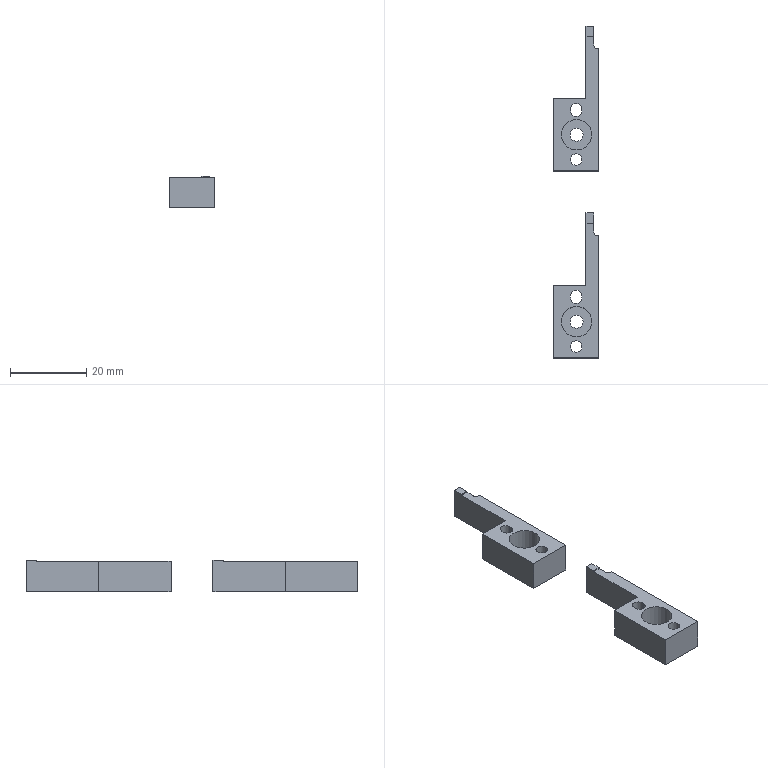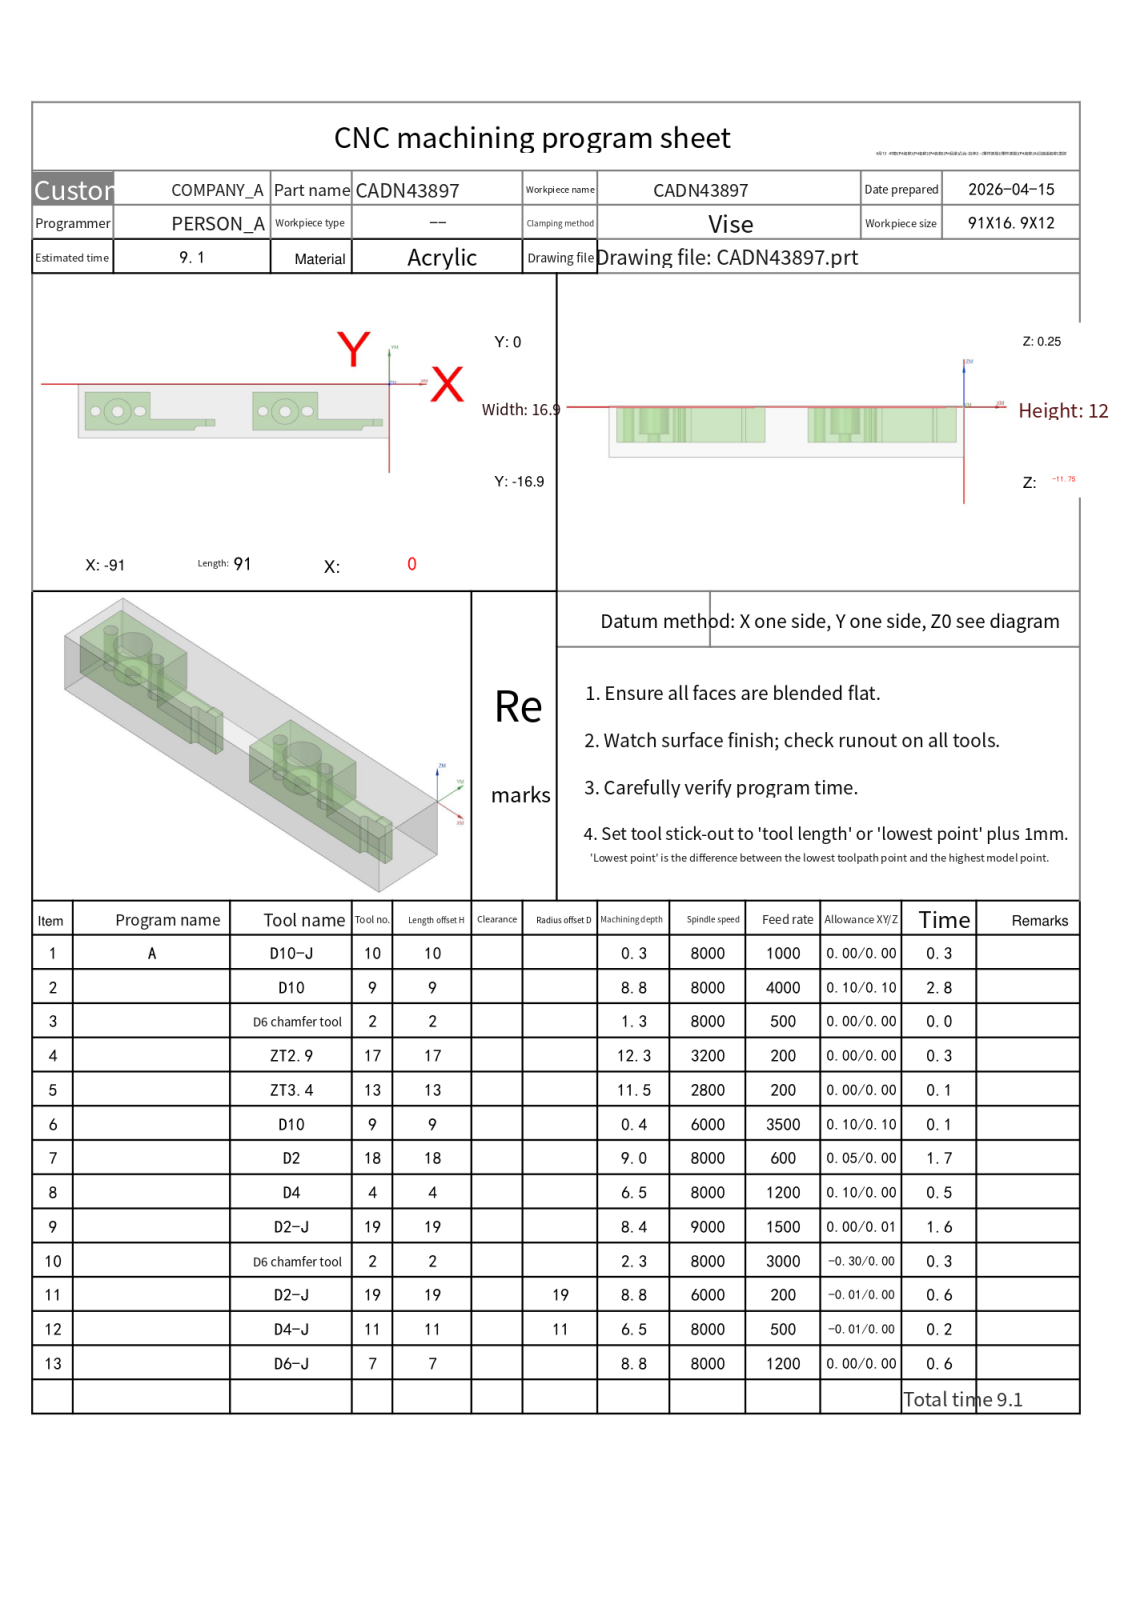NC program | NX | posted by the shop | part box 11.9 x 87 x 8.25 mm
Lines 2111 to 3431 of 9110, first 1079 of 1321 lines:
N7 T18 M06
(D2  D=2. R=0. H=18 ce=0.05 di=0.00)
G00 G90 G54 X-73. Y-8.05 M03 S6000
G43 H18 Z20.
M08
Z.25
G01 X-73.25 Z.244 F600.
G03 X-73.7 Y-8.5 Z.225 I0.0 J-.45
X-73.25 Y-8.95 Z.207 I.45 J0.0
G01 X-72.75 Z.194
G03 X-72.3 Y-8.5 Z.176 I0.0 J.45
X-72.75 Y-8.05 Z.158 I-.45 J0.0
G01 X-73.25 Z.145
G03 X-73.7 Y-8.5 Z.126 I0.0 J-.45
X-73.25 Y-8.95 Z.108 I.45 J0.0
G01 X-72.75 Z.095
G03 X-72.3 Y-8.5 Z.077 I0.0 J.45
X-72.75 Y-8.05 Z.059 I-.45 J0.0
G01 X-73.25 Z.046
G03 X-73.7 Y-8.5 Z.027 I0.0 J-.45
X-73.25 Y-8.95 Z.009 I.45 J0.0
G01 X-72.75 Z-.004
G03 X-72.3 Y-8.5 Z-.022 I0.0 J.45
X-72.75 Y-8.05 Z-.04 I-.45 J0.0
G01 X-73.25 Z-.053
G03 X-73.7 Y-8.5 Z-.071 I0.0 J-.45
X-73.25 Y-8.95 Z-.09 I.45 J0.0
G01 X-72.75 Z-.103
G03 X-72.3 Y-8.5 Z-.121 I0.0 J.45
X-72.75 Y-8.05 Z-.139 I-.45 J0.0
G01 X-73.25 Z-.152
G03 X-73.7 Y-8.5 Z-.17 I0.0 J-.45
X-73.25 Y-8.95 Z-.189 I.45 J0.0
G01 X-72.75 Z-.202
G03 X-72.3 Y-8.5 Z-.22 I0.0 J.45
X-72.75 Y-8.05 Z-.238 I-.45 J0.0
G01 X-73.25 Z-.251
G03 X-73.7 Y-8.5 Z-.269 I0.0 J-.45
X-73.25 Y-8.95 Z-.287 I.45 J0.0
G01 X-72.75 Z-.3
G03 X-72.3 Y-8.5 Z-.319 I0.0 J.45
X-72.75 Y-8.05 Z-.337 I-.45 J0.0
G01 X-73.25 Z-.35
G03 X-73.7 Y-8.5 Z-.368 I0.0 J-.45
X-73.25 Y-8.95 Z-.386 I.45 J0.0
G01 X-72.75 Z-.399
G03 X-72.3 Y-8.5 Z-.418 I0.0 J.45
X-72.75 Y-8.05 Z-.436 I-.45 J0.0
G01 X-73.25 Z-.449
G03 X-73.7 Y-8.5 Z-.467 I0.0 J-.45
X-73.25 Y-8.95 Z-.485 I.45 J0.0
G01 X-72.75 Z-.498
G03 X-72.3 Y-8.5 Z-.516 I0.0 J.45
X-72.75 Y-8.05 Z-.535 I-.45 J0.0
G01 X-73.25 Z-.548
G03 X-73.7 Y-8.5 Z-.566 I0.0 J-.45
X-73.25 Y-8.95 Z-.584 I.45 J0.0
G01 X-72.75 Z-.597
G03 X-72.3 Y-8.5 Z-.615 I0.0 J.45
X-72.75 Y-8.05 Z-.634 I-.45 J0.0
G01 X-73.25 Z-.647
G03 X-73.7 Y-8.5 Z-.665 I0.0 J-.45
X-73.25 Y-8.95 Z-.683 I.45 J0.0
G01 X-72.75 Z-.696
G03 X-72.3 Y-8.5 Z-.714 I0.0 J.45
X-72.75 Y-8.05 Z-.733 I-.45 J0.0
G01 X-73.25 Z-.745
G03 X-73.7 Y-8.5 Z-.764 I0.0 J-.45
X-73.25 Y-8.95 Z-.782 I.45 J0.0
G01 X-72.75 Z-.795
G03 X-72.3 Y-8.5 Z-.813 I0.0 J.45
X-72.75 Y-8.05 Z-.831 I-.45 J0.0
G01 X-73.25 Z-.844
G03 X-73.7 Y-8.5 Z-.863 I0.0 J-.45
X-73.25 Y-8.95 Z-.881 I.45 J0.0
G01 X-72.75 Z-.894
G03 X-72.3 Y-8.5 Z-.912 I0.0 J.45
X-72.75 Y-8.05 Z-.93 I-.45 J0.0
G01 X-73.25 Z-.943
G03 X-73.7 Y-8.5 Z-.962 I0.0 J-.45
X-73.25 Y-8.95 Z-.98 I.45 J0.0
G01 X-72.75 Z-.993
G03 X-72.3 Y-8.5 Z-1.011 I0.0 J.45
X-72.75 Y-8.05 Z-1.029 I-.45 J0.0
G01 X-73.25 Z-1.042
G03 X-73.7 Y-8.5 Z-1.06 I0.0 J-.45
X-73.25 Y-8.95 Z-1.079 I.45 J0.0
G01 X-72.75 Z-1.092
G03 X-72.3 Y-8.5 Z-1.11 I0.0 J.45
X-72.75 Y-8.05 Z-1.128 I-.45 J0.0
G01 X-73.25 Z-1.141
G03 X-73.7 Y-8.5 Z-1.159 I0.0 J-.45
X-73.25 Y-8.95 Z-1.178 I.45 J0.0
G01 X-72.75 Z-1.191
G03 X-72.3 Y-8.5 Z-1.209 I0.0 J.45
X-72.75 Y-8.05 Z-1.227 I-.45 J0.0
G01 X-73.25 Z-1.24
G03 X-73.7 Y-8.5 Z-1.258 I0.0 J-.45
X-73.25 Y-8.95 Z-1.277 I.45 J0.0
G01 X-72.75 Z-1.289
G03 X-72.3 Y-8.5 Z-1.308 I0.0 J.45
X-72.75 Y-8.05 Z-1.326 I-.45 J0.0
G01 X-73.25 Z-1.339
G03 X-73.7 Y-8.5 Z-1.357 I0.0 J-.45
X-73.25 Y-8.95 Z-1.375 I.45 J0.0
G01 X-72.75 Z-1.388
G03 X-72.3 Y-8.5 Z-1.407 I0.0 J.45
X-72.75 Y-8.05 Z-1.425 I-.45 J0.0
G01 X-73.25 Z-1.438
G03 X-73.7 Y-8.5 Z-1.456 I0.0 J-.45
X-73.25 Y-8.95 Z-1.474 I.45 J0.0
G01 X-72.75 Z-1.487
G03 X-72.3 Y-8.5 Z-1.505 I0.0 J.45
X-72.75 Y-8.05 Z-1.524 I-.45 J0.0
G01 X-73.25 Z-1.537
G03 X-73.7 Y-8.5 Z-1.555 I0.0 J-.45
X-73.25 Y-8.95 Z-1.573 I.45 J0.0
G01 X-72.75 Z-1.586
G03 X-72.3 Y-8.5 Z-1.604 I0.0 J.45
X-72.75 Y-8.05 Z-1.623 I-.45 J0.0
G01 X-73.25 Z-1.636
G03 X-73.7 Y-8.5 Z-1.654 I0.0 J-.45
X-73.25 Y-8.95 Z-1.672 I.45 J0.0
G01 X-72.75 Z-1.685
G03 X-72.3 Y-8.5 Z-1.703 I0.0 J.45
X-72.75 Y-8.05 Z-1.722 I-.45 J0.0
G01 X-73.25 Z-1.734
G03 X-73.7 Y-8.5 Z-1.753 I0.0 J-.45
X-73.25 Y-8.95 Z-1.771 I.45 J0.0
G01 X-72.75 Z-1.784
G03 X-72.3 Y-8.5 Z-1.802 I0.0 J.45
X-72.75 Y-8.05 Z-1.82 I-.45 J0.0
G01 X-73.25 Z-1.833
G03 X-73.7 Y-8.5 Z-1.852 I0.0 J-.45
X-73.25 Y-8.95 Z-1.87 I.45 J0.0
G01 X-72.75 Z-1.883
G03 X-72.3 Y-8.5 Z-1.901 I0.0 J.45
X-72.75 Y-8.05 Z-1.919 I-.45 J0.0
G01 X-73.25 Z-1.932
G03 X-73.7 Y-8.5 Z-1.951 I0.0 J-.45
X-73.25 Y-8.95 Z-1.969 I.45 J0.0
G01 X-72.75 Z-1.982
G03 X-72.3 Y-8.5 Z-2. I0.0 J.45
X-72.75 Y-8.05 Z-2.018 I-.45 J0.0
G01 X-73.25 Z-2.031
G03 X-73.7 Y-8.5 Z-2.049 I0.0 J-.45
X-73.25 Y-8.95 Z-2.068 I.45 J0.0
G01 X-72.75 Z-2.081
G03 X-72.3 Y-8.5 Z-2.099 I0.0 J.45
X-72.75 Y-8.05 Z-2.117 I-.45 J0.0
G01 X-73.25 Z-2.13
G03 X-73.7 Y-8.5 Z-2.148 I0.0 J-.45
X-73.25 Y-8.95 Z-2.167 I.45 J0.0
G01 X-72.75 Z-2.18
G03 X-72.3 Y-8.5 Z-2.198 I0.0 J.45
X-72.75 Y-8.05 Z-2.216 I-.45 J0.0
G01 X-73.25 Z-2.229
G03 X-73.7 Y-8.5 Z-2.247 I0.0 J-.45
X-73.25 Y-8.95 Z-2.266 I.45 J0.0
G01 X-72.75 Z-2.278
G03 X-72.3 Y-8.5 Z-2.297 I0.0 J.45
X-72.75 Y-8.05 Z-2.315 I-.45 J0.0
G01 X-73.25 Z-2.328
G03 X-73.7 Y-8.5 Z-2.346 I0.0 J-.45
X-73.25 Y-8.95 Z-2.364 I.45 J0.0
G01 X-72.75 Z-2.377
G03 X-72.3 Y-8.5 Z-2.396 I0.0 J.45
X-72.75 Y-8.05 Z-2.414 I-.45 J0.0
G01 X-73.25 Z-2.427
G03 X-73.7 Y-8.5 Z-2.445 I0.0 J-.45
X-73.25 Y-8.95 Z-2.463 I.45 J0.0
G01 X-72.75 Z-2.476
G03 X-72.3 Y-8.5 Z-2.495 I0.0 J.45
X-72.75 Y-8.05 Z-2.513 I-.45 J0.0
G01 X-73.25 Z-2.526
G03 X-73.7 Y-8.5 Z-2.544 I0.0 J-.45
X-73.25 Y-8.95 Z-2.562 I.45 J0.0
G01 X-72.75 Z-2.575
G03 X-72.3 Y-8.5 Z-2.593 I0.0 J.45
X-72.75 Y-8.05 Z-2.612 I-.45 J0.0
G01 X-73.25 Z-2.625
G03 X-73.7 Y-8.5 Z-2.643 I0.0 J-.45
X-73.25 Y-8.95 Z-2.661 I.45 J0.0
G01 X-72.75 Z-2.674
G03 X-72.3 Y-8.5 Z-2.692 I0.0 J.45
X-72.75 Y-8.05 Z-2.711 I-.45 J0.0
G01 X-73.25 Z-2.723
G03 X-73.7 Y-8.5 Z-2.742 I0.0 J-.45
X-73.25 Y-8.95 Z-2.76 I.45 J0.0
G01 X-72.75 Z-2.773
G03 X-72.3 Y-8.5 Z-2.791 I0.0 J.45
X-72.75 Y-8.05 Z-2.809 I-.45 J0.0
G01 X-73.25 Z-2.822
G03 X-73.7 Y-8.5 Z-2.841 I0.0 J-.45
X-73.25 Y-8.95 Z-2.859 I.45 J0.0
G01 X-72.75 Z-2.872
G03 X-72.3 Y-8.5 Z-2.89 I0.0 J.45
X-72.75 Y-8.05 Z-2.908 I-.45 J0.0
G01 X-73.25 Z-2.921
G03 X-73.7 Y-8.5 Z-2.94 I0.0 J-.45
X-73.25 Y-8.95 Z-2.958 I.45 J0.0
G01 X-72.75 Z-2.971
G03 X-72.3 Y-8.5 Z-2.989 I0.0 J.45
X-72.75 Y-8.05 Z-3.007 I-.45 J0.0
G01 X-73.25 Z-3.02
G03 X-73.7 Y-8.5 Z-3.038 I0.0 J-.45
X-73.25 Y-8.95 Z-3.057 I.45 J0.0
G01 X-72.75 Z-3.07
G03 X-72.3 Y-8.5 Z-3.088 I0.0 J.45
X-72.75 Y-8.05 Z-3.106 I-.45 J0.0
G01 X-73.25 Z-3.119
G03 X-73.7 Y-8.5 Z-3.137 I0.0 J-.45
X-73.25 Y-8.95 Z-3.156 I.45 J0.0
G01 X-72.75 Z-3.169
G03 X-72.3 Y-8.5 Z-3.187 I0.0 J.45
X-72.75 Y-8.05 Z-3.205 I-.45 J0.0
G01 X-73.25 Z-3.218
G03 X-73.7 Y-8.5 Z-3.236 I0.0 J-.45
X-73.25 Y-8.95 Z-3.255 I.45 J0.0
G01 X-72.75 Z-3.267
G03 X-72.3 Y-8.5 Z-3.286 I0.0 J.45
X-72.75 Y-8.05 Z-3.304 I-.45 J0.0
G01 X-73.25 Z-3.317
G03 X-73.7 Y-8.5 Z-3.335 I0.0 J-.45
X-73.25 Y-8.95 Z-3.353 I.45 J0.0
G01 X-72.75 Z-3.366
G03 X-72.3 Y-8.5 Z-3.385 I0.0 J.45
X-72.75 Y-8.05 Z-3.403 I-.45 J0.0
G01 X-73.25 Z-3.416
G03 X-73.7 Y-8.5 Z-3.434 I0.0 J-.45
X-73.25 Y-8.95 Z-3.452 I.45 J0.0
G01 X-72.75 Z-3.465
G03 X-72.3 Y-8.5 Z-3.484 I0.0 J.45
X-72.75 Y-8.05 Z-3.502 I-.45 J0.0
G01 X-73.25 Z-3.515
G03 X-73.7 Y-8.5 Z-3.533 I0.0 J-.45
X-73.25 Y-8.95 Z-3.551 I.45 J0.0
G01 X-72.75 Z-3.564
G03 X-72.3 Y-8.5 Z-3.582 I0.0 J.45
X-72.75 Y-8.05 Z-3.601 I-.45 J0.0
G01 X-73.25 Z-3.614
G03 X-73.7 Y-8.5 Z-3.632 I0.0 J-.45
X-73.25 Y-8.95 Z-3.65 I.45 J0.0
G01 X-72.75 Z-3.663
G03 X-72.3 Y-8.5 Z-3.681 I0.0 J.45
X-72.75 Y-8.05 Z-3.7 I-.45 J0.0
G01 X-73.25 Z-3.713
G03 X-73.7 Y-8.5 Z-3.731 I0.0 J-.45
X-73.25 Y-8.95 Z-3.749 I.45 J0.0
G01 X-72.75 Z-3.762
G03 X-72.3 Y-8.5 Z-3.78 I0.0 J.45
X-72.75 Y-8.05 Z-3.798 I-.45 J0.0
G01 X-73.25 Z-3.811
G03 X-73.7 Y-8.5 Z-3.83 I0.0 J-.45
X-73.25 Y-8.95 Z-3.848 I.45 J0.0
G01 X-72.75 Z-3.861
G03 X-72.3 Y-8.5 Z-3.879 I0.0 J.45
X-72.75 Y-8.05 Z-3.897 I-.45 J0.0
G01 X-73.25 Z-3.91
G03 X-73.7 Y-8.5 Z-3.929 I0.0 J-.45
X-73.25 Y-8.95 Z-3.947 I.45 J0.0
G01 X-72.75 Z-3.96
G03 X-72.3 Y-8.5 Z-3.978 I0.0 J.45
X-72.75 Y-8.05 Z-3.996 I-.45 J0.0
G01 X-73.25 Z-4.009
G03 X-73.7 Y-8.5 Z-4.027 I0.0 J-.45
X-73.25 Y-8.95 Z-4.046 I.45 J0.0
G01 X-72.75 Z-4.059
G03 X-72.3 Y-8.5 Z-4.077 I0.0 J.45
X-72.75 Y-8.05 Z-4.095 I-.45 J0.0
G01 X-73.25 Z-4.108
G03 X-73.7 Y-8.5 Z-4.126 I0.0 J-.45
X-73.25 Y-8.95 Z-4.145 I.45 J0.0
G01 X-72.75 Z-4.158
G03 X-72.3 Y-8.5 Z-4.176 I0.0 J.45
X-72.75 Y-8.05 Z-4.194 I-.45 J0.0
G01 X-73.25 Z-4.207
G03 X-73.7 Y-8.5 Z-4.225 I0.0 J-.45
X-73.25 Y-8.95 Z-4.244 I.45 J0.0
G01 X-72.75 Z-4.256
G03 X-72.3 Y-8.5 Z-4.275 I0.0 J.45
X-72.75 Y-8.05 Z-4.293 I-.45 J0.0
G01 X-73.25 Z-4.306
G03 X-73.7 Y-8.5 Z-4.324 I0.0 J-.45
X-73.25 Y-8.95 Z-4.342 I.45 J0.0
G01 X-72.75 Z-4.355
G03 X-72.3 Y-8.5 Z-4.374 I0.0 J.45
X-72.75 Y-8.05 Z-4.392 I-.45 J0.0
G01 X-73.25 Z-4.405
G03 X-73.7 Y-8.5 Z-4.423 I0.0 J-.45
X-73.25 Y-8.95 Z-4.441 I.45 J0.0
G01 X-72.75 Z-4.454
G03 X-72.3 Y-8.5 Z-4.473 I0.0 J.45
X-72.75 Y-8.05 Z-4.491 I-.45 J0.0
G01 X-73.25 Z-4.504
G03 X-73.7 Y-8.5 Z-4.522 I0.0 J-.45
X-73.25 Y-8.95 Z-4.54 I.45 J0.0
G01 X-72.75 Z-4.553
G03 X-72.3 Y-8.5 Z-4.571 I0.0 J.45
X-72.75 Y-8.05 Z-4.59 I-.45 J0.0
G01 X-73.25 Z-4.603
G03 X-73.7 Y-8.5 Z-4.621 I0.0 J-.45
X-73.25 Y-8.95 Z-4.639 I.45 J0.0
G01 X-72.75 Z-4.652
G03 X-72.3 Y-8.5 Z-4.67 I0.0 J.45
X-72.75 Y-8.05 Z-4.689 I-.45 J0.0
G01 X-73.25 Z-4.702
G03 X-73.7 Y-8.5 Z-4.72 I0.0 J-.45
X-73.25 Y-8.95 Z-4.738 I.45 J0.0
G01 X-72.75 Z-4.751
G03 X-72.3 Y-8.5 Z-4.769 I0.0 J.45
X-72.75 Y-8.05 Z-4.787 I-.45 J0.0
G01 X-73.25 Z-4.8
G03 X-73.7 Y-8.5 Z-4.819 I0.0 J-.45
X-73.25 Y-8.95 Z-4.837 I.45 J0.0
G01 X-72.75 Z-4.85
G03 X-72.3 Y-8.5 Z-4.868 I0.0 J.45
X-72.75 Y-8.05 Z-4.886 I-.45 J0.0
G01 X-73.25 Z-4.899
G03 X-73.7 Y-8.5 Z-4.918 I0.0 J-.45
X-73.25 Y-8.95 Z-4.936 I.45 J0.0
G01 X-72.75 Z-4.949
G03 X-72.3 Y-8.5 Z-4.967 I0.0 J.45
X-72.75 Y-8.05 Z-4.985 I-.45 J0.0
G01 X-73.25 Z-4.998
G03 X-73.7 Y-8.5 Z-5.016 I0.0 J-.45
X-73.25 Y-8.95 Z-5.035 I.45 J0.0
G01 X-72.75 Z-5.048
G03 X-72.3 Y-8.5 Z-5.066 I0.0 J.45
X-72.75 Y-8.05 Z-5.084 I-.45 J0.0
G01 X-73.25 Z-5.097
G03 X-73.7 Y-8.5 Z-5.115 I0.0 J-.45
X-73.25 Y-8.95 Z-5.134 I.45 J0.0
G01 X-72.75 Z-5.147
G03 X-72.3 Y-8.5 Z-5.165 I0.0 J.45
X-72.75 Y-8.05 Z-5.183 I-.45 J0.0
G01 X-73.25 Z-5.196
G03 X-73.7 Y-8.5 Z-5.214 I0.0 J-.45
X-73.25 Y-8.95 Z-5.233 I.45 J0.0
G01 X-72.75 Z-5.245
G03 X-72.3 Y-8.5 Z-5.264 I0.0 J.45
X-72.75 Y-8.05 Z-5.282 I-.45 J0.0
G01 X-73.25 Z-5.295
G03 X-73.7 Y-8.5 Z-5.313 I0.0 J-.45
X-73.25 Y-8.95 Z-5.331 I.45 J0.0
G01 X-72.75 Z-5.344
G03 X-72.3 Y-8.5 Z-5.363 I0.0 J.45
X-72.75 Y-8.05 Z-5.381 I-.45 J0.0
G01 X-73.25 Z-5.394
G03 X-73.7 Y-8.5 Z-5.412 I0.0 J-.45
X-73.25 Y-8.95 Z-5.43 I.45 J0.0
G01 X-72.75 Z-5.443
G03 X-72.3 Y-8.5 Z-5.462 I0.0 J.45
X-72.75 Y-8.05 Z-5.48 I-.45 J0.0
G01 X-73.25 Z-5.493
G03 X-73.7 Y-8.5 Z-5.511 I0.0 J-.45
X-73.25 Y-8.95 Z-5.529 I.45 J0.0
G01 X-72.75 Z-5.542
G03 X-72.3 Y-8.5 Z-5.56 I0.0 J.45
X-72.75 Y-8.05 Z-5.579 I-.45 J0.0
G01 X-73.25 Z-5.592
G03 X-73.7 Y-8.5 Z-5.61 I0.0 J-.45
X-73.25 Y-8.95 Z-5.628 I.45 J0.0
G01 X-72.75 Z-5.641
G03 X-72.3 Y-8.5 Z-5.659 I0.0 J.45
X-72.75 Y-8.05 Z-5.678 I-.45 J0.0
G01 X-73.25 Z-5.691
G03 X-73.7 Y-8.5 Z-5.709 I0.0 J-.45
X-73.25 Y-8.95 Z-5.727 I.45 J0.0
G01 X-72.75 Z-5.74
G03 X-72.3 Y-8.5 Z-5.758 I0.0 J.45
X-72.75 Y-8.05 Z-5.777 I-.45 J0.0
G01 X-73.25 Z-5.789
G03 X-73.7 Y-8.5 Z-5.808 I0.0 J-.45
X-73.25 Y-8.95 Z-5.826 I.45 J0.0
G01 X-72.75 Z-5.839
G03 X-72.3 Y-8.5 Z-5.857 I0.0 J.45
X-72.75 Y-8.05 Z-5.875 I-.45 J0.0
G01 X-73.25 Z-5.888
G03 X-73.7 Y-8.5 Z-5.907 I0.0 J-.45
X-73.25 Y-8.95 Z-5.925 I.45 J0.0
G01 X-72.75 Z-5.938
G03 X-72.3 Y-8.5 Z-5.956 I0.0 J.45
X-72.75 Y-8.05 Z-5.974 I-.45 J0.0
G01 X-73.25 Z-5.987
G03 X-73.7 Y-8.5 Z-6.005 I0.0 J-.45
X-73.25 Y-8.95 Z-6.024 I.45 J0.0
G01 X-72.75 Z-6.037
G03 X-72.3 Y-8.5 Z-6.055 I0.0 J.45
X-72.75 Y-8.05 Z-6.073 I-.45 J0.0
G01 X-73.25 Z-6.086
G03 X-73.7 Y-8.5 Z-6.104 I0.0 J-.45
X-73.25 Y-8.95 Z-6.123 I.45 J0.0
G01 X-72.75 Z-6.136
G03 X-72.3 Y-8.5 Z-6.154 I0.0 J.45
X-72.75 Y-8.05 Z-6.172 I-.45 J0.0
G01 X-73.25 Z-6.185
G03 X-73.7 Y-8.5 Z-6.203 I0.0 J-.45
X-73.25 Y-8.95 Z-6.222 I.45 J0.0
G01 X-72.75 Z-6.234
G03 X-72.3 Y-8.5 Z-6.253 I0.0 J.45
X-72.75 Y-8.05 Z-6.271 I-.45 J0.0
G01 X-73.25 Z-6.284
G03 X-73.7 Y-8.5 Z-6.302 I0.0 J-.45
X-73.25 Y-8.95 Z-6.32 I.45 J0.0
G01 X-72.75 Z-6.333
G03 X-72.3 Y-8.5 Z-6.352 I0.0 J.45
X-72.75 Y-8.05 Z-6.37 I-.45 J0.0
G01 X-73.25 Z-6.383
G03 X-73.7 Y-8.5 Z-6.401 I0.0 J-.45
X-73.25 Y-8.95 Z-6.419 I.45 J0.0
G01 X-72.75 Z-6.432
G03 X-72.3 Y-8.5 Z-6.451 I0.0 J.45
X-72.75 Y-8.05 Z-6.469 I-.45 J0.0
G01 X-73.25 Z-6.482
G03 X-73.7 Y-8.5 Z-6.5 I0.0 J-.45
X-73.25 Y-8.95 Z-6.518 I.45 J0.0
G01 X-72.75 Z-6.531
G03 X-72.3 Y-8.5 Z-6.549 I0.0 J.45
X-72.75 Y-8.05 Z-6.568 I-.45 J0.0
G01 X-73.25 Z-6.581
G03 X-73.7 Y-8.5 Z-6.599 I0.0 J-.45
X-73.25 Y-8.95 Z-6.617 I.45 J0.0
G01 X-72.75 Z-6.63
G03 X-72.3 Y-8.5 Z-6.648 I0.0 J.45
X-72.75 Y-8.05 Z-6.667 I-.45 J0.0
G01 X-73.25 Z-6.68
G03 X-73.7 Y-8.5 Z-6.698 I0.0 J-.45
X-73.25 Y-8.95 Z-6.716 I.45 J0.0
G01 X-72.75 Z-6.729
G03 X-72.3 Y-8.5 Z-6.747 I0.0 J.45
X-72.75 Y-8.05 Z-6.766 I-.45 J0.0
G01 X-73.25 Z-6.778
G03 X-73.7 Y-8.5 Z-6.797 I0.0 J-.45
X-73.25 Y-8.95 Z-6.815 I.45 J0.0
G01 X-72.75 Z-6.828
G03 X-72.3 Y-8.5 Z-6.846 I0.0 J.45
X-72.75 Y-8.05 Z-6.864 I-.45 J0.0
G01 X-73.25 Z-6.877
G03 X-73.7 Y-8.5 Z-6.896 I0.0 J-.45
X-73.25 Y-8.95 Z-6.914 I.45 J0.0
G01 X-72.75 Z-6.927
G03 X-72.3 Y-8.5 Z-6.945 I0.0 J.45
X-72.75 Y-8.05 Z-6.963 I-.45 J0.0
G01 X-73.25 Z-6.976
G03 X-73.7 Y-8.5 Z-6.995 I0.0 J-.45
X-73.25 Y-8.95 Z-7.013 I.45 J0.0
G01 X-72.75 Z-7.026
G03 X-72.3 Y-8.5 Z-7.044 I0.0 J.45
X-72.75 Y-8.05 Z-7.062 I-.45 J0.0
G01 X-73.25 Z-7.075
G03 X-73.7 Y-8.5 Z-7.093 I0.0 J-.45
X-73.25 Y-8.95 Z-7.112 I.45 J0.0
G01 X-72.75 Z-7.125
G03 X-72.3 Y-8.5 Z-7.143 I0.0 J.45
X-72.75 Y-8.05 Z-7.161 I-.45 J0.0
G01 X-73.25 Z-7.174
G03 X-73.7 Y-8.5 Z-7.192 I0.0 J-.45
X-73.25 Y-8.95 Z-7.211 I.45 J0.0
G01 X-72.75 Z-7.223
G03 X-72.3 Y-8.5 Z-7.242 I0.0 J.45
X-72.75 Y-8.05 Z-7.26 I-.45 J0.0
G01 X-73.25 Z-7.273
G03 X-73.7 Y-8.5 Z-7.291 I0.0 J-.45
X-73.25 Y-8.95 Z-7.309 I.45 J0.0
G01 X-72.75 Z-7.322
G03 X-72.3 Y-8.5 Z-7.341 I0.0 J.45
X-72.75 Y-8.05 Z-7.359 I-.45 J0.0
G01 X-73.25 Z-7.372
G03 X-73.7 Y-8.5 Z-7.39 I0.0 J-.45
X-73.25 Y-8.95 Z-7.408 I.45 J0.0
G01 X-72.75 Z-7.421
G03 X-72.3 Y-8.5 Z-7.44 I0.0 J.45
X-72.75 Y-8.05 Z-7.458 I-.45 J0.0
G01 X-73.25 Z-7.471
G03 X-73.7 Y-8.5 Z-7.489 I0.0 J-.45
X-73.25 Y-8.95 Z-7.507 I.45 J0.0
G01 X-72.75 Z-7.52
G03 X-72.3 Y-8.5 Z-7.538 I0.0 J.45
X-72.75 Y-8.05 Z-7.557 I-.45 J0.0
G01 X-73.25 Z-7.57
G03 X-73.7 Y-8.5 Z-7.588 I0.0 J-.45
X-73.25 Y-8.95 Z-7.606 I.45 J0.0
G01 X-72.75 Z-7.619
G03 X-72.3 Y-8.5 Z-7.637 I0.0 J.45
X-72.75 Y-8.05 Z-7.656 I-.45 J0.0
G01 X-73.25 Z-7.669
G03 X-73.7 Y-8.5 Z-7.687 I0.0 J-.45
X-73.25 Y-8.95 Z-7.705 I.45 J0.0
G01 X-72.75 Z-7.718
G03 X-72.3 Y-8.5 Z-7.736 I0.0 J.45
X-72.75 Y-8.05 Z-7.755 I-.45 J0.0
G01 X-73.25 Z-7.767
G03 X-73.7 Y-8.5 Z-7.786 I0.0 J-.45
X-73.25 Y-8.95 Z-7.804 I.45 J0.0
G01 X-72.75 Z-7.817
G03 X-72.3 Y-8.5 Z-7.835 I0.0 J.45
X-72.75 Y-8.05 Z-7.853 I-.45 J0.0
G01 X-73.25 Z-7.866
G03 X-73.7 Y-8.5 Z-7.885 I0.0 J-.45
X-73.25 Y-8.95 Z-7.903 I.45 J0.0
G01 X-72.75 Z-7.916
G03 X-72.3 Y-8.5 Z-7.934 I0.0 J.45
X-72.75 Y-8.05 Z-7.952 I-.45 J0.0
G01 X-73.25 Z-7.965
G03 X-73.7 Y-8.5 Z-7.984 I0.0 J-.45
X-73.25 Y-8.95 Z-8.002 I.45 J0.0
G01 X-72.75 Z-8.015
G03 X-72.3 Y-8.5 Z-8.033 I0.0 J.45
X-72.75 Y-8.05 Z-8.051 I-.45 J0.0
G01 X-73.25 Z-8.064
G03 X-73.7 Y-8.5 Z-8.082 I0.0 J-.45
X-73.25 Y-8.95 Z-8.101 I.45 J0.0
G01 X-72.75 Z-8.114
G03 X-72.3 Y-8.5 Z-8.132 I0.0 J.45
X-72.75 Y-8.05 Z-8.15 I-.45 J0.0
G01 X-73.25 Z-8.163
G03 X-73.7 Y-8.5 Z-8.181 I0.0 J-.45
X-73.25 Y-8.95 Z-8.2 I.45 J0.0
G01 X-72.75 Z-8.213
G03 X-72.3 Y-8.5 Z-8.231 I0.0 J.45
X-72.75 Y-8.05 Z-8.249 I-.45 J0.0
G01 X-73.25 Z-8.262
G03 X-73.7 Y-8.5 Z-8.28 I0.0 J-.45
X-73.25 Y-8.95 Z-8.298 I.45 J0.0
G01 X-72.75 Z-8.311
G03 X-72.3 Y-8.5 Z-8.33 I0.0 J.45
X-72.75 Y-8.05 Z-8.348 I-.45 J0.0
G01 X-73.25 Z-8.361
G03 X-73.7 Y-8.5 Z-8.379 I0.0 J-.45
X-73.25 Y-8.95 Z-8.397 I.45 J0.0
G01 X-72.75 Z-8.41
G03 X-72.3 Y-8.5 Z-8.429 I0.0 J.45
X-72.75 Y-8.05 Z-8.447 I-.45 J0.0
G01 X-73.25 Z-8.46
G03 X-73.7 Y-8.5 Z-8.478 I0.0 J-.45
X-73.25 Y-8.95 Z-8.496 I.45 J0.0
G01 X-72.75 Z-8.509
G03 X-72.3 Y-8.5 Z-8.527 I0.0 J.45
X-72.75 Y-8.05 Z-8.546 I-.45 J0.0
G01 X-73.25 Z-8.559
G03 X-73.7 Y-8.5 Z-8.577 I0.0 J-.45
X-73.25 Y-8.95 Z-8.595 I.45 J0.0
G01 X-72.75 Z-8.608
G03 X-72.3 Y-8.5 Z-8.626 I0.0 J.45
X-72.75 Y-8.05 Z-8.645 I-.45 J0.0
G01 X-73.25 Z-8.658
G03 X-73.7 Y-8.5 Z-8.676 I0.0 J-.45
X-73.25 Y-8.95 Z-8.694 I.45 J0.0
G01 X-72.75 Z-8.707
G03 X-72.3 Y-8.5 Z-8.725 I0.0 J.45
X-72.75 Y-8.05 Z-8.744 I-.45 J0.0
G01 X-73. Z-8.75
X-73.25
G03 X-73.7 Y-8.5 I0.0 J-.45
X-73.25 Y-8.95 I.45 J0.0
G01 X-72.75
G03 X-72.3 Y-8.5 I0.0 J.45
X-72.75 Y-8.05 I-.45 J0.0
G01 X-73.
X-73.25
G03 X-73.487 Y-8.118 I0.0 J-.45
G01 Z-7.75
G00 Z20.
X-24. Y-8.95
Z.25
G01 X-23.75 Z.244
G03 X-23.3 Y-8.5 Z.225 I0.0 J.45
X-23.75 Y-8.05 Z.207 I-.45 J0.0
G01 X-24.25 Z.194
G03 X-24.7 Y-8.5 Z.176 I0.0 J-.45
X-24.25 Y-8.95 Z.158 I.45 J0.0
G01 X-23.75 Z.145
G03 X-23.3 Y-8.5 Z.126 I0.0 J.45
X-23.75 Y-8.05 Z.108 I-.45 J0.0
G01 X-24.25 Z.095
G03 X-24.7 Y-8.5 Z.077 I0.0 J-.45
X-24.25 Y-8.95 Z.059 I.45 J0.0
G01 X-23.75 Z.046
G03 X-23.3 Y-8.5 Z.027 I0.0 J.45
X-23.75 Y-8.05 Z.009 I-.45 J0.0
G01 X-24.25 Z-.004
G03 X-24.7 Y-8.5 Z-.022 I0.0 J-.45
X-24.25 Y-8.95 Z-.04 I.45 J0.0
G01 X-23.75 Z-.053
G03 X-23.3 Y-8.5 Z-.071 I0.0 J.45
X-23.75 Y-8.05 Z-.09 I-.45 J0.0
G01 X-24.25 Z-.103
G03 X-24.7 Y-8.5 Z-.121 I0.0 J-.45
X-24.25 Y-8.95 Z-.139 I.45 J0.0
G01 X-23.75 Z-.152
G03 X-23.3 Y-8.5 Z-.17 I0.0 J.45
X-23.75 Y-8.05 Z-.189 I-.45 J0.0
G01 X-24.25 Z-.202
G03 X-24.7 Y-8.5 Z-.22 I0.0 J-.45
X-24.25 Y-8.95 Z-.238 I.45 J0.0
G01 X-23.75 Z-.251
G03 X-23.3 Y-8.5 Z-.269 I0.0 J.45
X-23.75 Y-8.05 Z-.287 I-.45 J0.0
G01 X-24.25 Z-.3
G03 X-24.7 Y-8.5 Z-.319 I0.0 J-.45
X-24.25 Y-8.95 Z-.337 I.45 J0.0
G01 X-23.75 Z-.35
G03 X-23.3 Y-8.5 Z-.368 I0.0 J.45
X-23.75 Y-8.05 Z-.386 I-.45 J0.0
G01 X-24.25 Z-.399
G03 X-24.7 Y-8.5 Z-.418 I0.0 J-.45
X-24.25 Y-8.95 Z-.436 I.45 J0.0
G01 X-23.75 Z-.449
G03 X-23.3 Y-8.5 Z-.467 I0.0 J.45
X-23.75 Y-8.05 Z-.485 I-.45 J0.0
G01 X-24.25 Z-.498
G03 X-24.7 Y-8.5 Z-.516 I0.0 J-.45
X-24.25 Y-8.95 Z-.535 I.45 J0.0
G01 X-23.75 Z-.548
G03 X-23.3 Y-8.5 Z-.566 I0.0 J.45
X-23.75 Y-8.05 Z-.584 I-.45 J0.0
G01 X-24.25 Z-.597
G03 X-24.7 Y-8.5 Z-.615 I0.0 J-.45
X-24.25 Y-8.95 Z-.634 I.45 J0.0
G01 X-23.75 Z-.647
G03 X-23.3 Y-8.5 Z-.665 I0.0 J.45
X-23.75 Y-8.05 Z-.683 I-.45 J0.0
G01 X-24.25 Z-.696
G03 X-24.7 Y-8.5 Z-.714 I0.0 J-.45
X-24.25 Y-8.95 Z-.733 I.45 J0.0
G01 X-23.75 Z-.745
G03 X-23.3 Y-8.5 Z-.764 I0.0 J.45
X-23.75 Y-8.05 Z-.782 I-.45 J0.0
G01 X-24.25 Z-.795
G03 X-24.7 Y-8.5 Z-.813 I0.0 J-.45
X-24.25 Y-8.95 Z-.831 I.45 J0.0
G01 X-23.75 Z-.844
G03 X-23.3 Y-8.5 Z-.863 I0.0 J.45
X-23.75 Y-8.05 Z-.881 I-.45 J0.0
G01 X-24.25 Z-.894
G03 X-24.7 Y-8.5 Z-.912 I0.0 J-.45
X-24.25 Y-8.95 Z-.93 I.45 J0.0
G01 X-23.75 Z-.943
G03 X-23.3 Y-8.5 Z-.962 I0.0 J.45
X-23.75 Y-8.05 Z-.98 I-.45 J0.0
G01 X-24.25 Z-.993
G03 X-24.7 Y-8.5 Z-1.011 I0.0 J-.45
X-24.25 Y-8.95 Z-1.029 I.45 J0.0
G01 X-23.75 Z-1.042
G03 X-23.3 Y-8.5 Z-1.06 I0.0 J.45
X-23.75 Y-8.05 Z-1.079 I-.45 J0.0
G01 X-24.25 Z-1.092
G03 X-24.7 Y-8.5 Z-1.11 I0.0 J-.45
X-24.25 Y-8.95 Z-1.128 I.45 J0.0
G01 X-23.75 Z-1.141
G03 X-23.3 Y-8.5 Z-1.159 I0.0 J.45
X-23.75 Y-8.05 Z-1.178 I-.45 J0.0
G01 X-24.25 Z-1.191
G03 X-24.7 Y-8.5 Z-1.209 I0.0 J-.45
X-24.25 Y-8.95 Z-1.227 I.45 J0.0
G01 X-23.75 Z-1.24
G03 X-23.3 Y-8.5 Z-1.258 I0.0 J.45
X-23.75 Y-8.05 Z-1.277 I-.45 J0.0
G01 X-24.25 Z-1.289
G03 X-24.7 Y-8.5 Z-1.308 I0.0 J-.45
X-24.25 Y-8.95 Z-1.326 I.45 J0.0
G01 X-23.75 Z-1.339
G03 X-23.3 Y-8.5 Z-1.357 I0.0 J.45
X-23.75 Y-8.05 Z-1.375 I-.45 J0.0
G01 X-24.25 Z-1.388
G03 X-24.7 Y-8.5 Z-1.407 I0.0 J-.45
X-24.25 Y-8.95 Z-1.425 I.45 J0.0
G01 X-23.75 Z-1.438
G03 X-23.3 Y-8.5 Z-1.456 I0.0 J.45
X-23.75 Y-8.05 Z-1.474 I-.45 J0.0
G01 X-24.25 Z-1.487
G03 X-24.7 Y-8.5 Z-1.505 I0.0 J-.45
X-24.25 Y-8.95 Z-1.524 I.45 J0.0
G01 X-23.75 Z-1.537
G03 X-23.3 Y-8.5 Z-1.555 I0.0 J.45
X-23.75 Y-8.05 Z-1.573 I-.45 J0.0
G01 X-24.25 Z-1.586
G03 X-24.7 Y-8.5 Z-1.604 I0.0 J-.45
X-24.25 Y-8.95 Z-1.623 I.45 J0.0
G01 X-23.75 Z-1.636
G03 X-23.3 Y-8.5 Z-1.654 I0.0 J.45
X-23.75 Y-8.05 Z-1.672 I-.45 J0.0
G01 X-24.25 Z-1.685
G03 X-24.7 Y-8.5 Z-1.703 I0.0 J-.45
X-24.25 Y-8.95 Z-1.722 I.45 J0.0
G01 X-23.75 Z-1.734
G03 X-23.3 Y-8.5 Z-1.753 I0.0 J.45
X-23.75 Y-8.05 Z-1.771 I-.45 J0.0
G01 X-24.25 Z-1.784
G03 X-24.7 Y-8.5 Z-1.802 I0.0 J-.45
X-24.25 Y-8.95 Z-1.82 I.45 J0.0
G01 X-23.75 Z-1.833
G03 X-23.3 Y-8.5 Z-1.852 I0.0 J.45
X-23.75 Y-8.05 Z-1.87 I-.45 J0.0
G01 X-24.25 Z-1.883
G03 X-24.7 Y-8.5 Z-1.901 I0.0 J-.45
X-24.25 Y-8.95 Z-1.919 I.45 J0.0
G01 X-23.75 Z-1.932
G03 X-23.3 Y-8.5 Z-1.951 I0.0 J.45
X-23.75 Y-8.05 Z-1.969 I-.45 J0.0
G01 X-24.25 Z-1.982
G03 X-24.7 Y-8.5 Z-2. I0.0 J-.45
X-24.25 Y-8.95 Z-2.018 I.45 J0.0
G01 X-23.75 Z-2.031
G03 X-23.3 Y-8.5 Z-2.049 I0.0 J.45
X-23.75 Y-8.05 Z-2.068 I-.45 J0.0
G01 X-24.25 Z-2.081
G03 X-24.7 Y-8.5 Z-2.099 I0.0 J-.45
X-24.25 Y-8.95 Z-2.117 I.45 J0.0
G01 X-23.75 Z-2.13
G03 X-23.3 Y-8.5 Z-2.148 I0.0 J.45
X-23.75 Y-8.05 Z-2.167 I-.45 J0.0
G01 X-24.25 Z-2.18
G03 X-24.7 Y-8.5 Z-2.198 I0.0 J-.45
X-24.25 Y-8.95 Z-2.216 I.45 J0.0
G01 X-23.75 Z-2.229
G03 X-23.3 Y-8.5 Z-2.247 I0.0 J.45
X-23.75 Y-8.05 Z-2.266 I-.45 J0.0
G01 X-24.25 Z-2.278
G03 X-24.7 Y-8.5 Z-2.297 I0.0 J-.45
X-24.25 Y-8.95 Z-2.315 I.45 J0.0
G01 X-23.75 Z-2.328
G03 X-23.3 Y-8.5 Z-2.346 I0.0 J.45
X-23.75 Y-8.05 Z-2.364 I-.45 J0.0
G01 X-24.25 Z-2.377
G03 X-24.7 Y-8.5 Z-2.396 I0.0 J-.45
X-24.25 Y-8.95 Z-2.414 I.45 J0.0
G01 X-23.75 Z-2.427
G03 X-23.3 Y-8.5 Z-2.445 I0.0 J.45
X-23.75 Y-8.05 Z-2.463 I-.45 J0.0
G01 X-24.25 Z-2.476
G03 X-24.7 Y-8.5 Z-2.495 I0.0 J-.45
X-24.25 Y-8.95 Z-2.513 I.45 J0.0
G01 X-23.75 Z-2.526
G03 X-23.3 Y-8.5 Z-2.544 I0.0 J.45
X-23.75 Y-8.05 Z-2.562 I-.45 J0.0
G01 X-24.25 Z-2.575
G03 X-24.7 Y-8.5 Z-2.593 I0.0 J-.45
X-24.25 Y-8.95 Z-2.612 I.45 J0.0
G01 X-23.75 Z-2.625
G03 X-23.3 Y-8.5 Z-2.643 I0.0 J.45
X-23.75 Y-8.05 Z-2.661 I-.45 J0.0
G01 X-24.25 Z-2.674
G03 X-24.7 Y-8.5 Z-2.692 I0.0 J-.45
X-24.25 Y-8.95 Z-2.711 I.45 J0.0
G01 X-23.75 Z-2.723
G03 X-23.3 Y-8.5 Z-2.742 I0.0 J.45
X-23.75 Y-8.05 Z-2.76 I-.45 J0.0
G01 X-24.25 Z-2.773
G03 X-24.7 Y-8.5 Z-2.791 I0.0 J-.45
X-24.25 Y-8.95 Z-2.809 I.45 J0.0
G01 X-23.75 Z-2.822
G03 X-23.3 Y-8.5 Z-2.841 I0.0 J.45
X-23.75 Y-8.05 Z-2.859 I-.45 J0.0
G01 X-24.25 Z-2.872
G03 X-24.7 Y-8.5 Z-2.89 I0.0 J-.45
X-24.25 Y-8.95 Z-2.908 I.45 J0.0
G01 X-23.75 Z-2.921
G03 X-23.3 Y-8.5 Z-2.94 I0.0 J.45
X-23.75 Y-8.05 Z-2.958 I-.45 J0.0
G01 X-24.25 Z-2.971
G03 X-24.7 Y-8.5 Z-2.989 I0.0 J-.45
X-24.25 Y-8.95 Z-3.007 I.45 J0.0
G01 X-23.75 Z-3.02
G03 X-23.3 Y-8.5 Z-3.038 I0.0 J.45
X-23.75 Y-8.05 Z-3.057 I-.45 J0.0
G01 X-24.25 Z-3.07
G03 X-24.7 Y-8.5 Z-3.088 I0.0 J-.45
X-24.25 Y-8.95 Z-3.106 I.45 J0.0
G01 X-23.75 Z-3.119
G03 X-23.3 Y-8.5 Z-3.137 I0.0 J.45
X-23.75 Y-8.05 Z-3.156 I-.45 J0.0
G01 X-24.25 Z-3.169
G03 X-24.7 Y-8.5 Z-3.187 I0.0 J-.45
X-24.25 Y-8.95 Z-3.205 I.45 J0.0
G01 X-23.75 Z-3.218
G03 X-23.3 Y-8.5 Z-3.236 I0.0 J.45
X-23.75 Y-8.05 Z-3.255 I-.45 J0.0
G01 X-24.25 Z-3.267
G03 X-24.7 Y-8.5 Z-3.286 I0.0 J-.45
X-24.25 Y-8.95 Z-3.304 I.45 J0.0
G01 X-23.75 Z-3.317
G03 X-23.3 Y-8.5 Z-3.335 I0.0 J.45
X-23.75 Y-8.05 Z-3.353 I-.45 J0.0
G01 X-24.25 Z-3.366
G03 X-24.7 Y-8.5 Z-3.385 I0.0 J-.45
X-24.25 Y-8.95 Z-3.403 I.45 J0.0
G01 X-23.75 Z-3.416
G03 X-23.3 Y-8.5 Z-3.434 I0.0 J.45
X-23.75 Y-8.05 Z-3.452 I-.45 J0.0
G01 X-24.25 Z-3.465
G03 X-24.7 Y-8.5 Z-3.484 I0.0 J-.45
X-24.25 Y-8.95 Z-3.502 I.45 J0.0
G01 X-23.75 Z-3.515
G03 X-23.3 Y-8.5 Z-3.533 I0.0 J.45
X-23.75 Y-8.05 Z-3.551 I-.45 J0.0
G01 X-24.25 Z-3.564
G03 X-24.7 Y-8.5 Z-3.582 I0.0 J-.45
X-24.25 Y-8.95 Z-3.601 I.45 J0.0
G01 X-23.75 Z-3.614
G03 X-23.3 Y-8.5 Z-3.632 I0.0 J.45
X-23.75 Y-8.05 Z-3.65 I-.45 J0.0
G01 X-24.25 Z-3.663
G03 X-24.7 Y-8.5 Z-3.681 I0.0 J-.45
X-24.25 Y-8.95 Z-3.7 I.45 J0.0
G01 X-23.75 Z-3.713
G03 X-23.3 Y-8.5 Z-3.731 I0.0 J.45
X-23.75 Y-8.05 Z-3.749 I-.45 J0.0
G01 X-24.25 Z-3.762
G03 X-24.7 Y-8.5 Z-3.78 I0.0 J-.45
X-24.25 Y-8.95 Z-3.798 I.45 J0.0
G01 X-23.75 Z-3.811
G03 X-23.3 Y-8.5 Z-3.83 I0.0 J.45
X-23.75 Y-8.05 Z-3.848 I-.45 J0.0
G01 X-24.25 Z-3.861
G03 X-24.7 Y-8.5 Z-3.879 I0.0 J-.45
X-24.25 Y-8.95 Z-3.897 I.45 J0.0
G01 X-23.75 Z-3.91
G03 X-23.3 Y-8.5 Z-3.929 I0.0 J.45
X-23.75 Y-8.05 Z-3.947 I-.45 J0.0
G01 X-24.25 Z-3.96
G03 X-24.7 Y-8.5 Z-3.978 I0.0 J-.45
X-24.25 Y-8.95 Z-3.996 I.45 J0.0
G01 X-23.75 Z-4.009
G03 X-23.3 Y-8.5 Z-4.027 I0.0 J.45
X-23.75 Y-8.05 Z-4.046 I-.45 J0.0
G01 X-24.25 Z-4.059
G03 X-24.7 Y-8.5 Z-4.077 I0.0 J-.45
X-24.25 Y-8.95 Z-4.095 I.45 J0.0
G01 X-23.75 Z-4.108
G03 X-23.3 Y-8.5 Z-4.126 I0.0 J.45
X-23.75 Y-8.05 Z-4.145 I-.45 J0.0
G01 X-24.25 Z-4.158
G03 X-24.7 Y-8.5 Z-4.176 I0.0 J-.45
X-24.25 Y-8.95 Z-4.194 I.45 J0.0
G01 X-23.75 Z-4.207
G03 X-23.3 Y-8.5 Z-4.225 I0.0 J.45
X-23.75 Y-8.05 Z-4.244 I-.45 J0.0
G01 X-24.25 Z-4.256
G03 X-24.7 Y-8.5 Z-4.275 I0.0 J-.45
X-24.25 Y-8.95 Z-4.293 I.45 J0.0
G01 X-23.75 Z-4.306
G03 X-23.3 Y-8.5 Z-4.324 I0.0 J.45
X-23.75 Y-8.05 Z-4.342 I-.45 J0.0
G01 X-24.25 Z-4.355
G03 X-24.7 Y-8.5 Z-4.374 I0.0 J-.45
X-24.25 Y-8.95 Z-4.392 I.45 J0.0
G01 X-23.75 Z-4.405
G03 X-23.3 Y-8.5 Z-4.423 I0.0 J.45
X-23.75 Y-8.05 Z-4.441 I-.45 J0.0
G01 X-24.25 Z-4.454
G03 X-24.7 Y-8.5 Z-4.473 I0.0 J-.45
X-24.25 Y-8.95 Z-4.491 I.45 J0.0
G01 X-23.75 Z-4.504
G03 X-23.3 Y-8.5 Z-4.522 I0.0 J.45
X-23.75 Y-8.05 Z-4.54 I-.45 J0.0
G01 X-24.25 Z-4.553
G03 X-24.7 Y-8.5 Z-4.571 I0.0 J-.45
X-24.25 Y-8.95 Z-4.59 I.45 J0.0
G01 X-23.75 Z-4.603
G03 X-23.3 Y-8.5 Z-4.621 I0.0 J.45
X-23.75 Y-8.05 Z-4.639 I-.45 J0.0
G01 X-24.25 Z-4.652
G03 X-24.7 Y-8.5 Z-4.67 I0.0 J-.45
X-24.25 Y-8.95 Z-4.689 I.45 J0.0
G01 X-23.75 Z-4.702
G03 X-23.3 Y-8.5 Z-4.72 I0.0 J.45
X-23.75 Y-8.05 Z-4.738 I-.45 J0.0
G01 X-24.25 Z-4.751
G03 X-24.7 Y-8.5 Z-4.769 I0.0 J-.45
X-24.25 Y-8.95 Z-4.787 I.45 J0.0
G01 X-23.75 Z-4.8
G03 X-23.3 Y-8.5 Z-4.819 I0.0 J.45
X-23.75 Y-8.05 Z-4.837 I-.45 J0.0
G01 X-24.25 Z-4.85
G03 X-24.7 Y-8.5 Z-4.868 I0.0 J-.45
X-24.25 Y-8.95 Z-4.886 I.45 J0.0
G01 X-23.75 Z-4.899
G03 X-23.3 Y-8.5 Z-4.918 I0.0 J.45
X-23.75 Y-8.05 Z-4.936 I-.45 J0.0
G01 X-24.25 Z-4.949
G03 X-24.7 Y-8.5 Z-4.967 I0.0 J-.45
X-24.25 Y-8.95 Z-4.985 I.45 J0.0
G01 X-23.75 Z-4.998
G03 X-23.3 Y-8.5 Z-5.016 I0.0 J.45
X-23.75 Y-8.05 Z-5.035 I-.45 J0.0
G01 X-24.25 Z-5.048
G03 X-24.7 Y-8.5 Z-5.066 I0.0 J-.45
X-24.25 Y-8.95 Z-5.084 I.45 J0.0
G01 X-23.75 Z-5.097
G03 X-23.3 Y-8.5 Z-5.115 I0.0 J.45
X-23.75 Y-8.05 Z-5.134 I-.45 J0.0
G01 X-24.25 Z-5.147
G03 X-24.7 Y-8.5 Z-5.165 I0.0 J-.45
X-24.25 Y-8.95 Z-5.183 I.45 J0.0
G01 X-23.75 Z-5.196
G03 X-23.3 Y-8.5 Z-5.214 I0.0 J.45
X-23.75 Y-8.05 Z-5.233 I-.45 J0.0
G01 X-24.25 Z-5.245
G03 X-24.7 Y-8.5 Z-5.264 I0.0 J-.45
X-24.25 Y-8.95 Z-5.282 I.45 J0.0
G01 X-23.75 Z-5.295
G03 X-23.3 Y-8.5 Z-5.313 I0.0 J.45
X-23.75 Y-8.05 Z-5.331 I-.45 J0.0
G01 X-24.25 Z-5.344
G03 X-24.7 Y-8.5 Z-5.363 I0.0 J-.45
X-24.25 Y-8.95 Z-5.381 I.45 J0.0
G01 X-23.75 Z-5.394
G03 X-23.3 Y-8.5 Z-5.412 I0.0 J.45
X-23.75 Y-8.05 Z-5.43 I-.45 J0.0
G01 X-24.25 Z-5.443
G03 X-24.7 Y-8.5 Z-5.462 I0.0 J-.45
X-24.25 Y-8.95 Z-5.48 I.45 J0.0
G01 X-23.75 Z-5.493
G03 X-23.3 Y-8.5 Z-5.511 I0.0 J.45
X-23.75 Y-8.05 Z-5.529 I-.45 J0.0
G01 X-24.25 Z-5.542
G03 X-24.7 Y-8.5 Z-5.56 I0.0 J-.45
X-24.25 Y-8.95 Z-5.579 I.45 J0.0
G01 X-23.75 Z-5.592
G03 X-23.3 Y-8.5 Z-5.61 I0.0 J.45
X-23.75 Y-8.05 Z-5.628 I-.45 J0.0
G01 X-24.25 Z-5.641
G03 X-24.7 Y-8.5 Z-5.659 I0.0 J-.45
X-24.25 Y-8.95 Z-5.678 I.45 J0.0
G01 X-23.75 Z-5.691
G03 X-23.3 Y-8.5 Z-5.709 I0.0 J.45
X-23.75 Y-8.05 Z-5.727 I-.45 J0.0
G01 X-24.25 Z-5.74
G03 X-24.7 Y-8.5 Z-5.758 I0.0 J-.45
X-24.25 Y-8.95 Z-5.777 I.45 J0.0
G01 X-23.75 Z-5.789
G03 X-23.3 Y-8.5 Z-5.808 I0.0 J.45
X-23.75 Y-8.05 Z-5.826 I-.45 J0.0
G01 X-24.25 Z-5.839
G03 X-24.7 Y-8.5 Z-5.857 I0.0 J-.45
X-24.25 Y-8.95 Z-5.875 I.45 J0.0
G01 X-23.75 Z-5.888
G03 X-23.3 Y-8.5 Z-5.907 I0.0 J.45
X-23.75 Y-8.05 Z-5.925 I-.45 J0.0
G01 X-24.25 Z-5.938
G03 X-24.7 Y-8.5 Z-5.956 I0.0 J-.45
X-24.25 Y-8.95 Z-5.974 I.45 J0.0
G01 X-23.75 Z-5.987
G03 X-23.3 Y-8.5 Z-6.005 I0.0 J.45
X-23.75 Y-8.05 Z-6.024 I-.45 J0.0
G01 X-24.25 Z-6.037
G03 X-24.7 Y-8.5 Z-6.055 I0.0 J-.45
X-24.25 Y-8.95 Z-6.073 I.45 J0.0
G01 X-23.75 Z-6.086
G03 X-23.3 Y-8.5 Z-6.104 I0.0 J.45
X-23.75 Y-8.05 Z-6.123 I-.45 J0.0
G01 X-24.25 Z-6.136
G03 X-24.7 Y-8.5 Z-6.154 I0.0 J-.45
X-24.25 Y-8.95 Z-6.172 I.45 J0.0
G01 X-23.75 Z-6.185
G03 X-23.3 Y-8.5 Z-6.203 I0.0 J.45
X-23.75 Y-8.05 Z-6.222 I-.45 J0.0
G01 X-24.25 Z-6.234
G03 X-24.7 Y-8.5 Z-6.253 I0.0 J-.45
X-24.25 Y-8.95 Z-6.271 I.45 J0.0
G01 X-23.75 Z-6.284
G03 X-23.3 Y-8.5 Z-6.302 I0.0 J.45
X-23.75 Y-8.05 Z-6.32 I-.45 J0.0
G01 X-24.25 Z-6.333
G03 X-24.7 Y-8.5 Z-6.352 I0.0 J-.45
X-24.25 Y-8.95 Z-6.37 I.45 J0.0
G01 X-23.75 Z-6.383
G03 X-23.3 Y-8.5 Z-6.401 I0.0 J.45
X-23.75 Y-8.05 Z-6.419 I-.45 J0.0
G01 X-24.25 Z-6.432
G03 X-24.7 Y-8.5 Z-6.451 I0.0 J-.45
X-24.25 Y-8.95 Z-6.469 I.45 J0.0
G01 X-23.75 Z-6.482
G03 X-23.3 Y-8.5 Z-6.5 I0.0 J.45
X-23.75 Y-8.05 Z-6.518 I-.45 J0.0
G01 X-24.25 Z-6.531
G03 X-24.7 Y-8.5 Z-6.549 I0.0 J-.45
X-24.25 Y-8.95 Z-6.568 I.45 J0.0
G01 X-23.75 Z-6.581
G03 X-23.3 Y-8.5 Z-6.599 I0.0 J.45
X-23.75 Y-8.05 Z-6.617 I-.45 J0.0
G01 X-24.25 Z-6.63
G03 X-24.7 Y-8.5 Z-6.648 I0.0 J-.45
X-24.25 Y-8.95 Z-6.667 I.45 J0.0
G01 X-23.75 Z-6.68
G03 X-23.3 Y-8.5 Z-6.698 I0.0 J.45
X-23.75 Y-8.05 Z-6.716 I-.45 J0.0
G01 X-24.25 Z-6.729
G03 X-24.7 Y-8.5 Z-6.747 I0.0 J-.45
X-24.25 Y-8.95 Z-6.766 I.45 J0.0
G01 X-23.75 Z-6.778
G03 X-23.3 Y-8.5 Z-6.797 I0.0 J.45
X-23.75 Y-8.05 Z-6.815 I-.45 J0.0
G01 X-24.25 Z-6.828
G03 X-24.7 Y-8.5 Z-6.846 I0.0 J-.45
X-24.25 Y-8.95 Z-6.864 I.45 J0.0
G01 X-23.75 Z-6.877
G03 X-23.3 Y-8.5 Z-6.896 I0.0 J.45
X-23.75 Y-8.05 Z-6.914 I-.45 J0.0
G01 X-24.25 Z-6.927
G03 X-24.7 Y-8.5 Z-6.945 I0.0 J-.45
X-24.25 Y-8.95 Z-6.963 I.45 J0.0
G01 X-23.75 Z-6.976
G03 X-23.3 Y-8.5 Z-6.995 I0.0 J.45
X-23.75 Y-8.05 Z-7.013 I-.45 J0.0
G01 X-24.25 Z-7.026
G03 X-24.7 Y-8.5 Z-7.044 I0.0 J-.45
X-24.25 Y-8.95 Z-7.062 I.45 J0.0
G01 X-23.75 Z-7.075
G03 X-23.3 Y-8.5 Z-7.093 I0.0 J.45
X-23.75 Y-8.05 Z-7.112 I-.45 J0.0
G01 X-24.25 Z-7.125
G03 X-24.7 Y-8.5 Z-7.143 I0.0 J-.45
X-24.25 Y-8.95 Z-7.161 I.45 J0.0
G01 X-23.75 Z-7.174
G03 X-23.3 Y-8.5 Z-7.192 I0.0 J.45
X-23.75 Y-8.05 Z-7.211 I-.45 J0.0
G01 X-24.25 Z-7.223
G03 X-24.7 Y-8.5 Z-7.242 I0.0 J-.45
X-24.25 Y-8.95 Z-7.26 I.45 J0.0
G01 X-23.75 Z-7.273
G03 X-23.3 Y-8.5 Z-7.291 I0.0 J.45
X-23.75 Y-8.05 Z-7.309 I-.45 J0.0
G01 X-24.25 Z-7.322
G03 X-24.7 Y-8.5 Z-7.341 I0.0 J-.45
X-24.25 Y-8.95 Z-7.359 I.45 J0.0
G01 X-23.75 Z-7.372
G03 X-23.3 Y-8.5 Z-7.39 I0.0 J.45
X-23.75 Y-8.05 Z-7.408 I-.45 J0.0
G01 X-24.25 Z-7.421
G03 X-24.7 Y-8.5 Z-7.44 I0.0 J-.45
X-24.25 Y-8.95 Z-7.458 I.45 J0.0
G01 X-23.75 Z-7.471
G03 X-23.3 Y-8.5 Z-7.489 I0.0 J.45
X-23.75 Y-8.05 Z-7.507 I-.45 J0.0
G01 X-24.25 Z-7.52
G03 X-24.7 Y-8.5 Z-7.538 I0.0 J-.45
X-24.25 Y-8.95 Z-7.557 I.45 J0.0
G01 X-23.75 Z-7.57
G03 X-23.3 Y-8.5 Z-7.588 I0.0 J.45
X-23.75 Y-8.05 Z-7.606 I-.45 J0.0
G01 X-24.25 Z-7.619
G03 X-24.7 Y-8.5 Z-7.637 I0.0 J-.45
X-24.25 Y-8.95 Z-7.656 I.45 J0.0
G01 X-23.75 Z-7.669
G03 X-23.3 Y-8.5 Z-7.687 I0.0 J.45
X-23.75 Y-8.05 Z-7.705 I-.45 J0.0
G01 X-24.25 Z-7.718
G03 X-24.7 Y-8.5 Z-7.736 I0.0 J-.45
X-24.25 Y-8.95 Z-7.755 I.45 J0.0
G01 X-23.75 Z-7.767
G03 X-23.3 Y-8.5 Z-7.786 I0.0 J.45
X-23.75 Y-8.05 Z-7.804 I-.45 J0.0
G01 X-24.25 Z-7.817
G03 X-24.7 Y-8.5 Z-7.835 I0.0 J-.45
X-24.25 Y-8.95 Z-7.853 I.45 J0.0
G01 X-23.75 Z-7.866
G03 X-23.3 Y-8.5 Z-7.885 I0.0 J.45
X-23.75 Y-8.05 Z-7.903 I-.45 J0.0
G01 X-24.25 Z-7.916
G03 X-24.7 Y-8.5 Z-7.934 I0.0 J-.45
X-24.25 Y-8.95 Z-7.952 I.45 J0.0
G01 X-23.75 Z-7.965
G03 X-23.3 Y-8.5 Z-7.984 I0.0 J.45
X-23.75 Y-8.05 Z-8.002 I-.45 J0.0
G01 X-24.25 Z-8.015
G03 X-24.7 Y-8.5 Z-8.033 I0.0 J-.45
X-24.25 Y-8.95 Z-8.051 I.45 J0.0
G01 X-23.75 Z-8.064
G03 X-23.3 Y-8.5 Z-8.082 I0.0 J.45
X-23.75 Y-8.05 Z-8.101 I-.45 J0.0
G01 X-24.25 Z-8.114
G03 X-24.7 Y-8.5 Z-8.132 I0.0 J-.45
X-24.25 Y-8.95 Z-8.15 I.45 J0.0
G01 X-23.75 Z-8.163
G03 X-23.3 Y-8.5 Z-8.181 I0.0 J.45
X-23.75 Y-8.05 Z-8.2 I-.45 J0.0